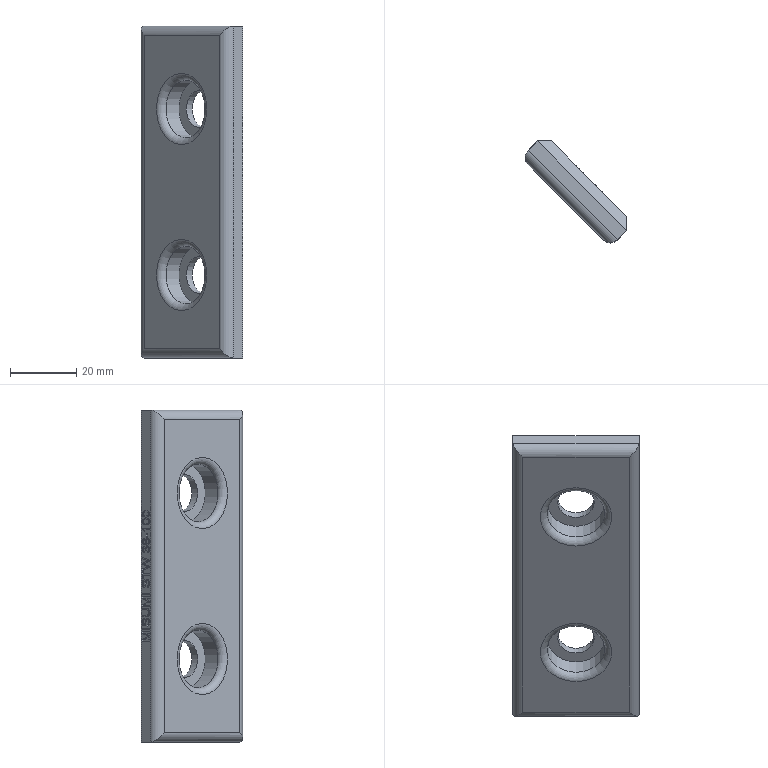Part | NX | features solid 2 | 1 solid | 147 faces | box 30.577 x 30.577 x 100 mm | volume 32082 mm3 | plane 95 | spline 42 | cylinder 8 | torus 2 | commonest cylinder face diameters 6 x4 11.007 x2 17.5 x2